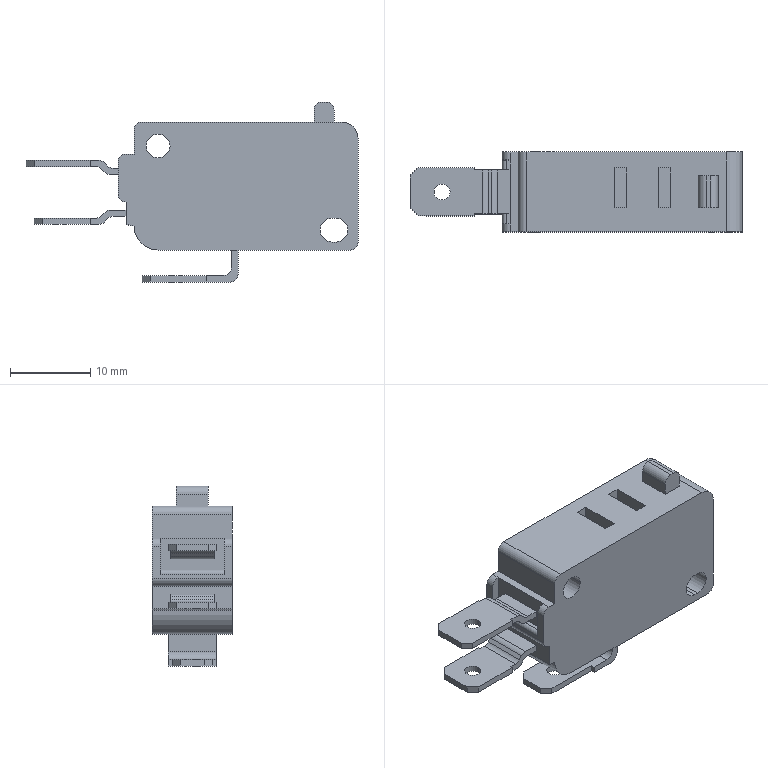Part | Creo | 1 solid | 104 faces | box 41.5 x 10 x 22.5 mm | volume 4526 mm3 | plane 74 | cylinder 30 | commonest cylinder face diameters 2 x23 3 x4 1 x1 4 x1 6 x1